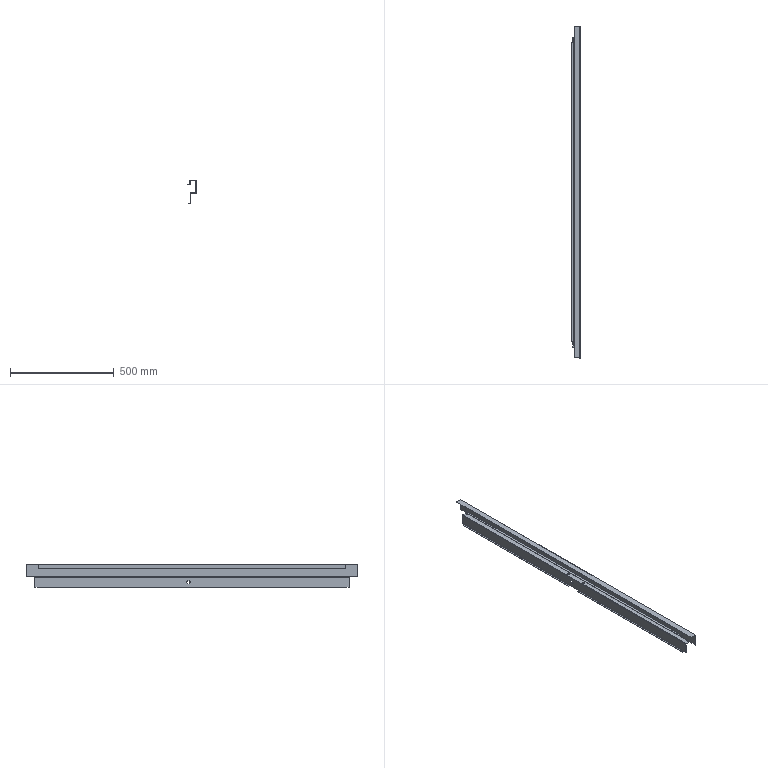Part | STEP file | 1 solid | 96 faces | box 40.001 x 1598 x 110 mm | volume 311237 mm3 | plane 73 | cylinder 23 | commonest cylinder face diameters 0.4 x7 2.4 x6 6.1 x4 9 x4 16 x2